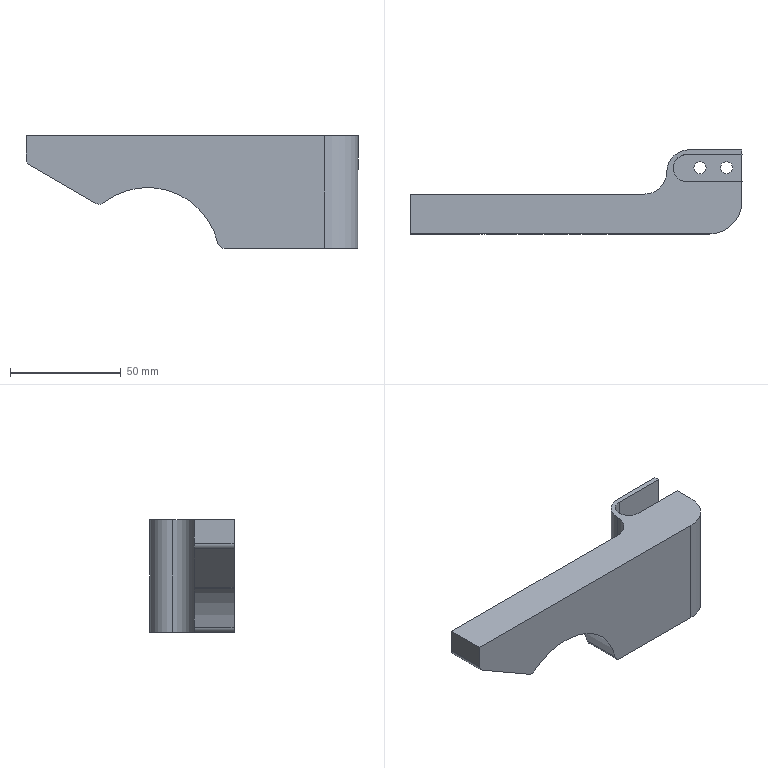NC program | NX | posted with a generic post | part box 150 x 38 x 51 mm
Lines 4517 to 4810 of 31037:
(ZLEVEL_PROFILE_COPY_COPY_COPY_1_COPY_COPY_COPY , TOOL : D12JING)
N9002 T11 M6
N9004 G54
N9006 G17 G0 G90 X-77.569 Y28.25 S9500 M3
N9008 G43 Z30. H11
N9010 Z-12.75
N9012 G94 G1 X-76.039 Y25.6 F1000.
N9014 G3 X-75. Y25. R1.2
N9016 G1 X60. F1200.
N9018 G2 X81. Y4. R21.
N9020 G1 Y-19.
N9022 G2 X75. Y-25. R6.
N9024 G1 X51.
N9026 G2 X35. Y-9. R16.
N9028 G3 X31. Y-5. R4.
N9030 G1 X-75.
N9032 G2 X-81. Y1.002 R6.
N9034 G1 Y19.001
N9036 G2 X-75. Y25. R6.
N9038 G3 X-73.961 Y25.6 R1.2
N9040 G1 X-72.229 Y28.6
N9042 G0 X-77.569 Y28.25 Z-25.5
N9044 G1 X-76.039 Y25.6 F1000.
N9046 G3 X-75. Y25. R1.2
N9048 G1 X60. F1200.
N9050 G2 X81. Y4. R21.
N9052 G1 Y-19.
N9054 G2 X75. Y-25. R6.
N9056 G1 X51.
N9058 G2 X35. Y-9. R16.
N9060 G3 X31. Y-5. R4.
N9062 G1 X-75.
N9064 G2 X-81. Y1.002 R6.
N9066 G1 Y19.001
N9068 G2 X-75. Y25. R6.
N9070 G3 X-73.961 Y25.6 R1.2
N9072 G1 X-72.229 Y28.6
N9074 G0 X-77.569 Y28.25 Z-38.25
N9076 G1 X-76.039 Y25.6 F1000.
N9078 G3 X-75. Y25. R1.2
N9080 G1 X60. F1200.
N9082 G2 X81. Y4. R21.
N9084 G1 Y-19.
N9086 G2 X75. Y-25. R6.
N9088 G1 X51.
N9090 G2 X35. Y-9. R16.
N9092 G3 X31. Y-5. R4.
N9094 G1 X-75.
N9096 G2 X-81. Y1.002 R6.
N9098 G1 Y19.001
N9100 G2 X-75. Y25. R6.
N9102 G3 X-73.961 Y25.6 R1.2
N9104 G1 X-72.229 Y28.6
N9106 G0 X-77.569 Y28.25 Z-51.
N9108 G1 X-76.039 Y25.6 F1000.
N9110 G3 X-75. Y25. R1.2
N9112 G1 X60. F1200.
N9114 G2 X81. Y4. R21.
N9116 G1 Y-19.
N9118 G2 X75. Y-25. R6.
N9120 G1 X51.
N9122 G2 X35. Y-9. R16.
N9124 G3 X31. Y-5. R4.
N9126 G1 X-75.
N9128 G2 X-81. Y1.002 R6.
N9130 G1 Y19.001
N9132 G2 X-75. Y25. R6.
N9134 G3 X-73.961 Y25.6 R1.2
N9136 G1 X-72.229 Y28.6
N9138 G0 Z30.
N9140 M5
(HOLE_MILLING , TOOL : D6)
N9142 T06 M6
N9144 G54
N9146 G17 G0 G90 X56. Y-10.9 S9500 M3
N9148 G43 Z30. H6
N9150 Z0.5
N9152 G94 G3 X57.375 Y-12.275 R1.375 F850.
N9154 X58.75 Y-10.9 R1.375
N9156 X58.75 Y-10.9 Z0.15 I-2.75 J0.
N9158 X58.75 Y-10.9 Z-0.2 I-2.75 J0.
N9160 X58.75 Y-10.9 Z-0.55 I-2.75 J0.
N9162 X58.75 Y-10.9 Z-0.9 I-2.75 J0.
N9164 X58.75 Y-10.9 Z-1.25 I-2.75 J0.
N9166 X58.75 Y-10.9 Z-1.6 I-2.75 J0.
N9168 X58.75 Y-10.9 Z-1.95 I-2.75 J0.
N9170 X58.75 Y-10.9 Z-2.3 I-2.75 J0.
N9172 X58.75 Y-10.9 Z-2.65 I-2.75 J0.
N9174 X58.75 Y-10.9 Z-3. I-2.75 J0.
N9176 X58.75 Y-10.9 Z-3.35 I-2.75 J0.
N9178 X58.75 Y-10.9 Z-3.7 I-2.75 J0.
N9180 X58.75 Y-10.9 Z-4.05 I-2.75 J0.
N9182 X58.75 Y-10.9 Z-4.4 I-2.75 J0.
N9184 X58.75 Y-10.9 Z-4.75 I-2.75 J0.
N9186 X58.75 Y-10.9 Z-5.1 I-2.75 J0.
N9188 X58.75 Y-10.9 Z-5.45 I-2.75 J0.
N9190 X58.75 Y-10.9 Z-5.8 I-2.75 J0.
N9192 X58.75 Y-10.9 Z-6.15 I-2.75 J0.
N9194 X58.75 Y-10.9 Z-6.5 I-2.75 J0.
N9196 X58.75 Y-10.9 Z-6.85 I-2.75 J0.
N9198 X58.75 Y-10.9 Z-7.2 I-2.75 J0.
N9200 X58.75 Y-10.9 Z-7.55 I-2.75 J0.
N9202 X58.75 Y-10.9 Z-7.9 I-2.75 J0.
N9204 X58.75 Y-10.9 Z-8.25 I-2.75 J0.
N9206 X58.75 Y-10.9 Z-8.6 I-2.75 J0.
N9208 X58.75 Y-10.9 Z-8.95 I-2.75 J0.
N9210 X58.75 Y-10.9 Z-9.3 I-2.75 J0.
N9212 X58.75 Y-10.9 Z-9.65 I-2.75 J0.
N9214 X58.75 Y-10.9 Z-10. I-2.75 J0.
N9216 X58.75 Y-10.9 Z-10.35 I-2.75 J0.
N9218 X58.75 Y-10.9 Z-10.7 I-2.75 J0.
N9220 X58.75 Y-10.9 Z-11.05 I-2.75 J0.
N9222 X58.75 Y-10.9 Z-11.4 I-2.75 J0.
N9224 X58.75 Y-10.9 Z-11.75 I-2.75 J0.
N9226 X58.75 Y-10.9 Z-12.1 I-2.75 J0.
N9228 X58.75 Y-10.9 Z-12.45 I-2.75 J0.
N9230 X58.75 Y-10.9 Z-12.8 I-2.75 J0.
N9232 X58.75 Y-10.9 Z-13.15 I-2.75 J0.
N9234 X58.75 Y-10.9 Z-13.5 I-2.75 J0.
N9236 X58.75 Y-10.9 Z-13.85 I-2.75 J0.
N9238 X58.75 Y-10.9 Z-14.2 I-2.75 J0.
N9240 X58.75 Y-10.9 Z-14.55 I-2.75 J0.
N9242 X58.75 Y-10.9 Z-14.9 I-2.75 J0.
N9244 X58.75 Y-10.9 Z-15.25 I-2.75 J0.
N9246 X58.75 Y-10.9 Z-15.6 I-2.75 J0.
N9248 X58.75 Y-10.9 Z-15.95 I-2.75 J0.
N9250 X58.75 Y-10.9 Z-16.3 I-2.75 J0.
N9252 X58.75 Y-10.9 Z-16.65 I-2.75 J0.
N9254 X58.75 Y-10.9 Z-17. I-2.75 J0.
N9256 X58.75 Y-10.9 Z-17.35 I-2.75 J0.
N9258 X58.75 Y-10.9 Z-17.7 I-2.75 J0.
N9260 X58.75 Y-10.9 Z-18.05 I-2.75 J0.
N9262 X58.75 Y-10.9 Z-18.4 I-2.75 J0.
N9264 X58.75 Y-10.9 Z-18.75 I-2.75 J0.
N9266 X58.75 Y-10.9 Z-19.1 I-2.75 J0.
N9268 X58.75 Y-10.9 Z-19.45 I-2.75 J0.
N9270 X58.75 Y-10.9 Z-19.8 I-2.75 J0.
N9272 X58.75 Y-10.9 Z-20.15 I-2.75 J0.
N9274 X58.75 Y-10.9 Z-20.5 I-2.75 J0.
N9276 X58.75 Y-10.9 Z-20.85 I-2.75 J0.
N9278 X58.75 Y-10.9 Z-21.2 I-2.75 J0.
N9280 X58.75 Y-10.9 Z-21.55 I-2.75 J0.
N9282 X58.75 Y-10.9 Z-21.9 I-2.75 J0.
N9284 X58.75 Y-10.9 Z-22.25 I-2.75 J0.
N9286 X58.75 Y-10.9 Z-22.6 I-2.75 J0.
N9288 X58.75 Y-10.9 Z-22.95 I-2.75 J0.
N9290 X58.75 Y-10.9 Z-23.3 I-2.75 J0.
N9292 X58.75 Y-10.9 Z-23.65 I-2.75 J0.
N9294 X58.75 Y-10.9 Z-24. I-2.75 J0.
N9296 X58.75 Y-10.9 Z-24.35 I-2.75 J0.
N9298 X58.75 Y-10.9 Z-24.7 I-2.75 J0.
N9300 X58.75 Y-10.9 Z-25.05 I-2.75 J0.
N9302 X58.75 Y-10.9 Z-25.4 I-2.75 J0.
N9304 X58.75 Y-10.9 Z-25.75 I-2.75 J0.
N9306 X57.715 Y-8.75 Z-25.8 R2.75
N9308 X53.85 Y-9.185 R2.75
N9310 X57.715 Y-8.75 R-2.75
N9312 X55.782 Y-8.968 R1.375
N9314 X56. Y-10.9 R1.375
N9316 G0 Z30.
N9318 X68.
N9320 Z0.5
N9322 G3 X69.375 Y-12.275 R1.375
N9324 X70.75 Y-10.9 R1.375
N9326 X70.75 Y-10.9 Z0.15 I-2.75 J0.
N9328 X70.75 Y-10.9 Z-0.2 I-2.75 J0.
N9330 X70.75 Y-10.9 Z-0.55 I-2.75 J0.
N9332 X70.75 Y-10.9 Z-0.9 I-2.75 J0.
N9334 X70.75 Y-10.9 Z-1.25 I-2.75 J0.
N9336 X70.75 Y-10.9 Z-1.6 I-2.75 J0.
N9338 X70.75 Y-10.9 Z-1.95 I-2.75 J0.
N9340 X70.75 Y-10.9 Z-2.3 I-2.75 J0.
N9342 X70.75 Y-10.9 Z-2.65 I-2.75 J0.
N9344 X70.75 Y-10.9 Z-3. I-2.75 J0.
N9346 X70.75 Y-10.9 Z-3.35 I-2.75 J0.
N9348 X70.75 Y-10.9 Z-3.7 I-2.75 J0.
N9350 X70.75 Y-10.9 Z-4.05 I-2.75 J0.
N9352 X70.75 Y-10.9 Z-4.4 I-2.75 J0.
N9354 X70.75 Y-10.9 Z-4.75 I-2.75 J0.
N9356 X70.75 Y-10.9 Z-5.1 I-2.75 J0.
N9358 X70.75 Y-10.9 Z-5.45 I-2.75 J0.
N9360 X70.75 Y-10.9 Z-5.8 I-2.75 J0.
N9362 X70.75 Y-10.9 Z-6.15 I-2.75 J0.
N9364 X70.75 Y-10.9 Z-6.5 I-2.75 J0.
N9366 X70.75 Y-10.9 Z-6.85 I-2.75 J0.
N9368 X70.75 Y-10.9 Z-7.2 I-2.75 J0.
N9370 X70.75 Y-10.9 Z-7.55 I-2.75 J0.
N9372 X70.75 Y-10.9 Z-7.9 I-2.75 J0.
N9374 X70.75 Y-10.9 Z-8.25 I-2.75 J0.
N9376 X70.75 Y-10.9 Z-8.6 I-2.75 J0.
N9378 X70.75 Y-10.9 Z-8.95 I-2.75 J0.
N9380 X70.75 Y-10.9 Z-9.3 I-2.75 J0.
N9382 X70.75 Y-10.9 Z-9.65 I-2.75 J0.
N9384 X70.75 Y-10.9 Z-10. I-2.75 J0.
N9386 X70.75 Y-10.9 Z-10.35 I-2.75 J0.
N9388 X70.75 Y-10.9 Z-10.7 I-2.75 J0.
N9390 X70.75 Y-10.9 Z-11.05 I-2.75 J0.
N9392 X70.75 Y-10.9 Z-11.4 I-2.75 J0.
N9394 X70.75 Y-10.9 Z-11.75 I-2.75 J0.
N9396 X70.75 Y-10.9 Z-12.1 I-2.75 J0.
N9398 X70.75 Y-10.9 Z-12.45 I-2.75 J0.
N9400 X70.75 Y-10.9 Z-12.8 I-2.75 J0.
N9402 X70.75 Y-10.9 Z-13.15 I-2.75 J0.
N9404 X70.75 Y-10.9 Z-13.5 I-2.75 J0.
N9406 X70.75 Y-10.9 Z-13.85 I-2.75 J0.
N9408 X70.75 Y-10.9 Z-14.2 I-2.75 J0.
N9410 X70.75 Y-10.9 Z-14.55 I-2.75 J0.
N9412 X70.75 Y-10.9 Z-14.9 I-2.75 J0.
N9414 X70.75 Y-10.9 Z-15.25 I-2.75 J0.
N9416 X70.75 Y-10.9 Z-15.6 I-2.75 J0.
N9418 X70.75 Y-10.9 Z-15.95 I-2.75 J0.
N9420 X70.75 Y-10.9 Z-16.3 I-2.75 J0.
N9422 X70.75 Y-10.9 Z-16.65 I-2.75 J0.
N9424 X70.75 Y-10.9 Z-17. I-2.75 J0.
N9426 X70.75 Y-10.9 Z-17.35 I-2.75 J0.
N9428 X70.75 Y-10.9 Z-17.7 I-2.75 J0.
N9430 X70.75 Y-10.9 Z-18.05 I-2.75 J0.
N9432 X70.75 Y-10.9 Z-18.4 I-2.75 J0.
N9434 X70.75 Y-10.9 Z-18.75 I-2.75 J0.
N9436 X70.75 Y-10.9 Z-19.1 I-2.75 J0.
N9438 X70.75 Y-10.9 Z-19.45 I-2.75 J0.
N9440 X70.75 Y-10.9 Z-19.8 I-2.75 J0.
N9442 X70.75 Y-10.9 Z-20.15 I-2.75 J0.
N9444 X70.75 Y-10.9 Z-20.5 I-2.75 J0.
N9446 X70.75 Y-10.9 Z-20.85 I-2.75 J0.
N9448 X70.75 Y-10.9 Z-21.2 I-2.75 J0.
N9450 X70.75 Y-10.9 Z-21.55 I-2.75 J0.
N9452 X70.75 Y-10.9 Z-21.9 I-2.75 J0.
N9454 X70.75 Y-10.9 Z-22.25 I-2.75 J0.
N9456 X70.75 Y-10.9 Z-22.6 I-2.75 J0.
N9458 X70.75 Y-10.9 Z-22.95 I-2.75 J0.
N9460 X70.75 Y-10.9 Z-23.3 I-2.75 J0.
N9462 X70.75 Y-10.9 Z-23.65 I-2.75 J0.
N9464 X70.75 Y-10.9 Z-24. I-2.75 J0.
N9466 X70.75 Y-10.9 Z-24.35 I-2.75 J0.
N9468 X70.75 Y-10.9 Z-24.7 I-2.75 J0.
N9470 X70.75 Y-10.9 Z-25.05 I-2.75 J0.
N9472 X70.75 Y-10.9 Z-25.4 I-2.75 J0.
N9474 X70.75 Y-10.9 Z-25.75 I-2.75 J0.
N9476 X69.715 Y-8.75 Z-25.8 R2.75
N9478 X65.85 Y-9.185 R2.75
N9480 X69.715 Y-8.75 R-2.75
N9482 X67.782 Y-8.968 R1.375
N9484 X68. Y-10.9 R1.375
N9486 G0 Z30.
N9488 M5
(PLANAR_MILL , TOOL : D6A45)
N9490 T07 M6
N9492 G54
N9494 G17 G0 G90 X72.133 Y-11.891 S9500 M3
N9496 G43 Z30. H7
N9498 Z0.
N9500 G94 G1 Z-1. F1250.
N9502 X72.35 Y-11.766
N9504 G3 X72.85 Y-10.9 R1.
N9506 X68. Y-6.05 R4.85
N9508 X72.85 Y-10.9 R-4.85
N9510 X72.35 Y-10.034 R1.
N9512 G1 X72.133 Y-9.909
N9514 Z0.
N9516 G0 Z30.
N9518 X55.009 Y-15.033
N9520 Z0.
N9522 G1 Z-1.
N9524 X55.134 Y-15.25
N9526 G3 X56. Y-15.75 R1.
N9528 X60.85 Y-10.9 R4.85
N9530 X56. Y-15.75 R-4.85
N9532 X56.866 Y-15.25 R1.
N9534 G1 X56.991 Y-15.033
N9536 Z0.
N9538 G0 Z30.
N9540 X15.635 Y20.818
N9542 Z0.
N9544 G1 Z-1.
N9546 G3 X15.783 Y19.9 R1.
N9548 G1 X60.
N9550 G2 X75.9 Y4. R15.9
N9552 G1 Y-18.9
N9554 G2 X74.9 Y-19.9 R1.
N9556 G1 X51.
N9558 G2 X40.1 Y-9. R10.9
N9560 G3 X31. Y0.1 R9.1
N9562 G1 X15.783
N9564 G3 X15.635 Y-0.818 R1.
N9566 G1 Z0.
N9568 G0 Z30.
N9570 M5